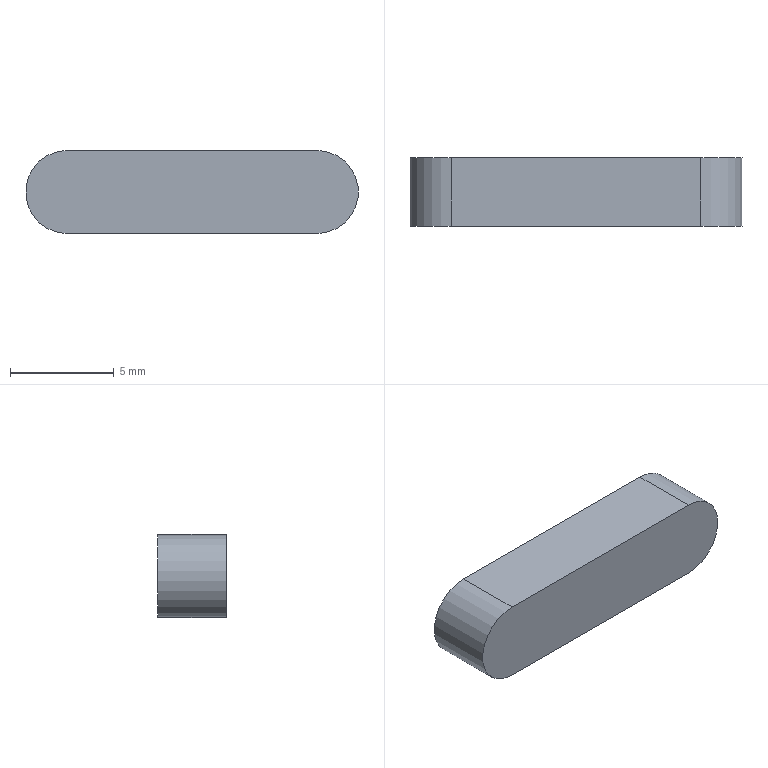Part | NX | features BREP 1 | 1 solid | 6 faces | box 16 x 3.3 x 4 mm | volume 199.869 mm3 | plane 4 | cylinder 2 | commonest cylinder face diameters 4 x2
STEP:
#1=CARTESIAN_POINT('',(0.,0.,-2.));
#2=VERTEX_POINT('',#1);
#3=CARTESIAN_POINT('',(0.,0.,2.));
#4=VERTEX_POINT('',#3);
#5=CARTESIAN_POINT('',(0.,0.,0.));
#6=DIRECTION('',(0.,1.,0.));
#7=DIRECTION('',(0.,0.,1.));
#8=AXIS2_PLACEMENT_3D('',#5,#6,#7);
#9=CIRCLE('',#8,2.);
#10=EDGE_CURVE('',#2,#4,#9,.T.);
#11=ORIENTED_EDGE('',*,*,#10,.T.);
#12=CARTESIAN_POINT('',(0.,3.3,2.));
#13=VERTEX_POINT('',#12);
#14=CARTESIAN_POINT('',(0.,3.3,2.));
#15=DIRECTION('',(0.,-1.,0.));
#16=VECTOR('',#15,1000.);
#17=LINE('',#14,#16);
#18=EDGE_CURVE('',#13,#4,#17,.T.);
#19=ORIENTED_EDGE('',*,*,#18,.F.);
#20=CARTESIAN_POINT('',(0.,3.3,-2.));
#21=VERTEX_POINT('',#20);
#22=CARTESIAN_POINT('',(0.,3.3,0.));
#23=DIRECTION('',(0.,1.,0.));
#24=DIRECTION('',(0.,0.,1.));
#25=AXIS2_PLACEMENT_3D('',#22,#23,#24);
#26=CIRCLE('',#25,2.);
#27=EDGE_CURVE('',#21,#13,#26,.T.);
#28=ORIENTED_EDGE('',*,*,#27,.F.);
#29=CARTESIAN_POINT('',(0.,3.3,-2.));
#30=DIRECTION('',(0.,-1.,0.));
#31=VECTOR('',#30,1000.);
#32=LINE('',#29,#31);
#33=EDGE_CURVE('',#21,#2,#32,.T.);
#34=ORIENTED_EDGE('',*,*,#33,.T.);
#35=EDGE_LOOP('',(#11,#19,#28,#34));
#36=FACE_BOUND('',#35,.T.);
#37=CARTESIAN_POINT('',(0.,3.3,0.));
#38=DIRECTION('',(0.,-1.,0.));
#39=DIRECTION('',(0.,0.,1.));
#40=AXIS2_PLACEMENT_3D('',#37,#38,#39);
#41=CYLINDRICAL_SURFACE('',#40,2.);
#42=ADVANCED_FACE('',(#36),#41,.T.);
#43=CARTESIAN_POINT('',(12.,0.,2.));
#44=VERTEX_POINT('',#43);
#45=CARTESIAN_POINT('',(0.,0.,2.));
#46=DIRECTION('',(1.,0.,0.));
#47=VECTOR('',#46,1000.);
#48=LINE('',#45,#47);
#49=EDGE_CURVE('',#4,#44,#48,.T.);
#50=ORIENTED_EDGE('',*,*,#49,.T.);
#51=CARTESIAN_POINT('',(12.,3.3,2.));
#52=VERTEX_POINT('',#51);
#53=CARTESIAN_POINT('',(12.,3.3,2.));
#54=DIRECTION('',(0.,-1.,0.));
#55=VECTOR('',#54,1000.);
#56=LINE('',#53,#55);
#57=EDGE_CURVE('',#52,#44,#56,.T.);
#58=ORIENTED_EDGE('',*,*,#57,.F.);
#59=CARTESIAN_POINT('',(0.,3.3,2.));
#60=DIRECTION('',(1.,0.,0.));
#61=VECTOR('',#60,1000.);
#62=LINE('',#59,#61);
#63=EDGE_CURVE('',#13,#52,#62,.T.);
#64=ORIENTED_EDGE('',*,*,#63,.F.);
#65=ORIENTED_EDGE('',*,*,#18,.T.);
#66=EDGE_LOOP('',(#50,#58,#64,#65));
#67=FACE_BOUND('',#66,.T.);
#68=CARTESIAN_POINT('',(0.,3.3,2.));
#69=DIRECTION('',(0.,0.,-1.));
#70=DIRECTION('',(1.,0.,0.));
#71=AXIS2_PLACEMENT_3D('',#68,#69,#70);
#72=PLANE('',#71);
#73=ADVANCED_FACE('',(#67),#72,.F.);
#74=CARTESIAN_POINT('',(12.,0.,-2.));
#75=VERTEX_POINT('',#74);
#76=CARTESIAN_POINT('',(12.,0.,0.));
#77=DIRECTION('',(0.,1.,0.));
#78=DIRECTION('',(0.,0.,1.));
#79=AXIS2_PLACEMENT_3D('',#76,#77,#78);
#80=CIRCLE('',#79,2.);
#81=EDGE_CURVE('',#44,#75,#80,.T.);
#82=ORIENTED_EDGE('',*,*,#81,.T.);
#83=CARTESIAN_POINT('',(12.,3.3,-2.));
#84=VERTEX_POINT('',#83);
#85=CARTESIAN_POINT('',(12.,3.3,-2.));
#86=DIRECTION('',(0.,-1.,0.));
#87=VECTOR('',#86,1000.);
#88=LINE('',#85,#87);
#89=EDGE_CURVE('',#84,#75,#88,.T.);
#90=ORIENTED_EDGE('',*,*,#89,.F.);
#91=CARTESIAN_POINT('',(12.,3.3,0.));
#92=DIRECTION('',(0.,1.,0.));
#93=DIRECTION('',(0.,0.,1.));
#94=AXIS2_PLACEMENT_3D('',#91,#92,#93);
#95=CIRCLE('',#94,2.);
#96=EDGE_CURVE('',#52,#84,#95,.T.);
#97=ORIENTED_EDGE('',*,*,#96,.F.);
#98=ORIENTED_EDGE('',*,*,#57,.T.);
#99=EDGE_LOOP('',(#82,#90,#97,#98));
#100=FACE_BOUND('',#99,.T.);
#101=CARTESIAN_POINT('',(12.,3.3,0.));
#102=DIRECTION('',(0.,-1.,0.));
#103=DIRECTION('',(0.,0.,1.));
#104=AXIS2_PLACEMENT_3D('',#101,#102,#103);
#105=CYLINDRICAL_SURFACE('',#104,2.);
#106=ADVANCED_FACE('',(#100),#105,.T.);
#107=CARTESIAN_POINT('',(0.,0.,-2.));
#108=DIRECTION('',(-1.,0.,0.));
#109=VECTOR('',#108,1000.);
#110=LINE('',#107,#109);
#111=EDGE_CURVE('',#75,#2,#110,.T.);
#112=ORIENTED_EDGE('',*,*,#111,.T.);
#113=ORIENTED_EDGE('',*,*,#33,.F.);
#114=CARTESIAN_POINT('',(0.,3.3,-2.));
#115=DIRECTION('',(-1.,0.,0.));
#116=VECTOR('',#115,1000.);
#117=LINE('',#114,#116);
#118=EDGE_CURVE('',#84,#21,#117,.T.);
#119=ORIENTED_EDGE('',*,*,#118,.F.);
#120=ORIENTED_EDGE('',*,*,#89,.T.);
#121=EDGE_LOOP('',(#112,#113,#119,#120));
#122=FACE_BOUND('',#121,.T.);
#123=CARTESIAN_POINT('',(0.,3.3,-2.));
#124=DIRECTION('',(0.,0.,1.));
#125=DIRECTION('',(0.,1.,0.));
#126=AXIS2_PLACEMENT_3D('',#123,#124,#125);
#127=PLANE('',#126);
#128=ADVANCED_FACE('',(#122),#127,.F.);
#129=ORIENTED_EDGE('',*,*,#27,.T.);
#130=ORIENTED_EDGE('',*,*,#63,.T.);
#131=ORIENTED_EDGE('',*,*,#96,.T.);
#132=ORIENTED_EDGE('',*,*,#118,.T.);
#133=EDGE_LOOP('',(#129,#130,#131,#132));
#134=FACE_BOUND('',#133,.T.);
#135=CARTESIAN_POINT('',(0.,3.3,0.));
#136=DIRECTION('',(0.,1.,0.));
#137=DIRECTION('',(0.,0.,1.));
#138=AXIS2_PLACEMENT_3D('',#135,#136,#137);
#139=PLANE('',#138);
#140=ADVANCED_FACE('',(#134),#139,.T.);
#141=ORIENTED_EDGE('',*,*,#10,.F.);
#142=ORIENTED_EDGE('',*,*,#111,.F.);
#143=ORIENTED_EDGE('',*,*,#81,.F.);
#144=ORIENTED_EDGE('',*,*,#49,.F.);
#145=EDGE_LOOP('',(#141,#142,#143,#144));
#146=FACE_BOUND('',#145,.T.);
#147=CARTESIAN_POINT('',(0.,0.,0.));
#148=DIRECTION('',(0.,1.,0.));
#149=DIRECTION('',(0.,0.,1.));
#150=AXIS2_PLACEMENT_3D('',#147,#148,#149);
#151=PLANE('',#150);
#152=ADVANCED_FACE('',(#146),#151,.F.);
#153=CLOSED_SHELL('',(#42,#73,#106,#128,#140,#152));
#154=MANIFOLD_SOLID_BREP('',#153);
#155=(LENGTH_UNIT()NAMED_UNIT(*)SI_UNIT(.MILLI.,.METRE.));
#156=UNCERTAINTY_MEASURE_WITH_UNIT(LENGTH_MEASURE(0.00001),#155,'','');
#157=(NAMED_UNIT(*)PLANE_ANGLE_UNIT()SI_UNIT($,.RADIAN.));
#158=(NAMED_UNIT(*)SI_UNIT($,.STERADIAN.)SOLID_ANGLE_UNIT());
#159=(GEOMETRIC_REPRESENTATION_CONTEXT(3)GLOBAL_UNCERTAINTY_ASSIGNED_CONTEXT((#156))GLOBAL_UNIT_ASSIGNED_CONTEXT((#155,#157,#158))REPRESENTATION_CONTEXT('',''));
#160=ADVANCED_BREP_SHAPE_REPRESENTATION('',(#154),#159);